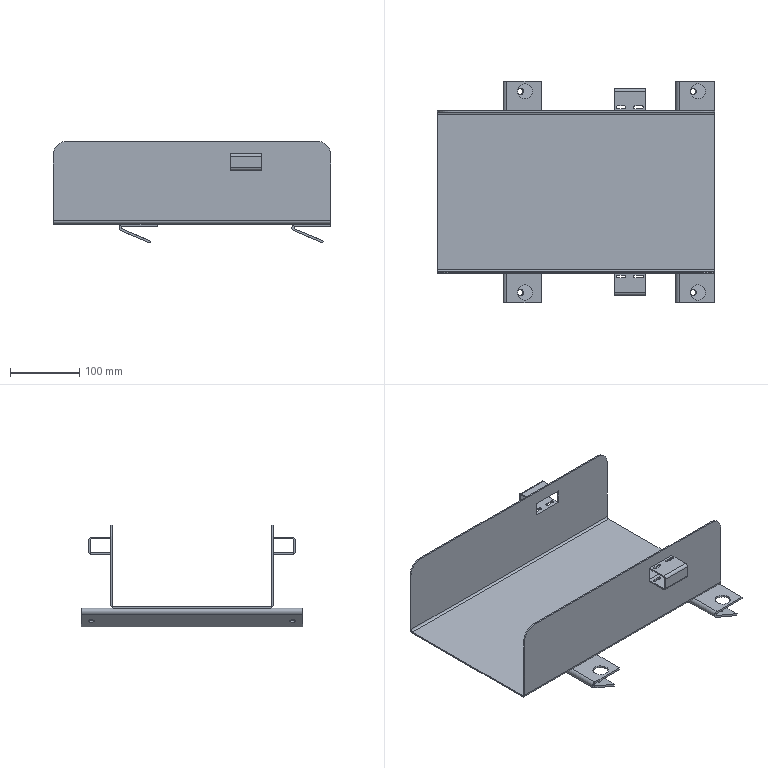Part | STEP file | NG chute L | 1 solid | 124 faces | box 400 x 320 x 147.024 mm | volume 579162 mm3 | plane 64 | cylinder 60 | commonest cylinder face diameters 4 x30 9 x8 22 x8 8 x4 10 x4 40 x4